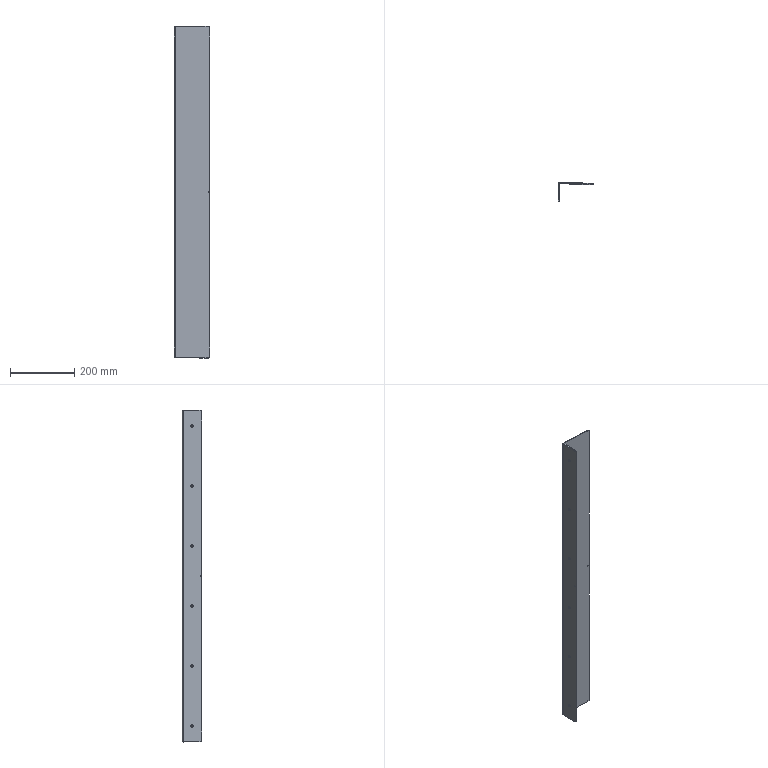Part | STEP file | TS-018-01 | 1 solid | 42 faces | box 109.914 x 59.871 x 1030 mm | volume 512009 mm3 | plane 28 | cylinder 14 | commonest cylinder face diameters 8 x12 0.4 x1 6.4 x1